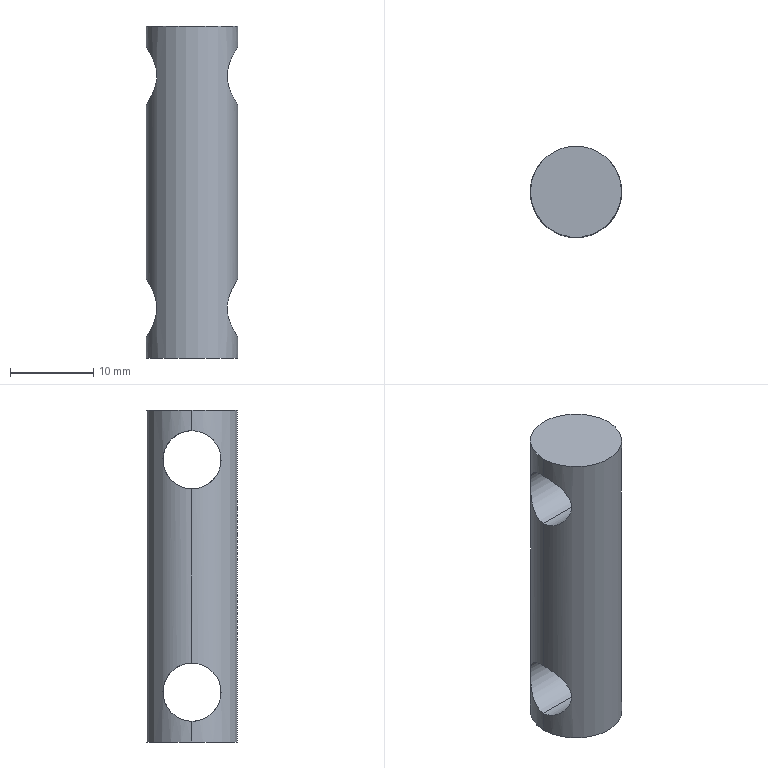Part | SolidWorks | features Extrusion 1, ICE 1 | 1 solid | 8 faces | box 11 x 11 x 40 mm | volume 3000 mm3 | cylinder 6 | plane 2 | commonest cylinder face diameters 7 x4 11 x2
STEP:
#1=CARTESIAN_POINT('',(-5.5,0.,-10.5));
#2=VERTEX_POINT('',#1);
#3=CARTESIAN_POINT('',(-5.5,0.,-17.5));
#4=VERTEX_POINT('',#3);
#5=CARTESIAN_POINT('',(-5.5,0.,-10.5));
#6=CARTESIAN_POINT('',(-5.5,-0.2386,-10.5));
#7=CARTESIAN_POINT('',(-5.485,-0.472,-10.524));
#8=CARTESIAN_POINT('',(-5.426,-0.9292,-10.618));
#9=CARTESIAN_POINT('',(-5.382,-1.155,-10.688));
#10=CARTESIAN_POINT('',(-5.219,-1.788,-10.957));
#11=CARTESIAN_POINT('',(-5.067,-2.167,-11.216));
#12=CARTESIAN_POINT('',(-4.83,-2.636,-11.687));
#13=CARTESIAN_POINT('',(-4.748,-2.779,-11.861));
#14=CARTESIAN_POINT('',(-4.594,-3.028,-12.231));
#15=CARTESIAN_POINT('',(-4.521,-3.134,-12.426));
#16=CARTESIAN_POINT('',(-4.393,-3.311,-12.843));
#17=CARTESIAN_POINT('',(-4.338,-3.381,-13.067));
#18=CARTESIAN_POINT('',(-4.263,-3.475,-13.523));
#19=CARTESIAN_POINT('',(-4.243,-3.5,-13.76));
#20=CARTESIAN_POINT('',(-4.242,-3.5,-14.234));
#21=CARTESIAN_POINT('',(-4.262,-3.477,-14.467));
#22=CARTESIAN_POINT('',(-4.337,-3.383,-14.926));
#23=CARTESIAN_POINT('',(-4.391,-3.314,-15.148));
#24=CARTESIAN_POINT('',(-4.519,-3.137,-15.568));
#25=CARTESIAN_POINT('',(-4.593,-3.029,-15.768));
#26=CARTESIAN_POINT('',(-4.748,-2.78,-16.138));
#27=CARTESIAN_POINT('',(-4.829,-2.639,-16.31));
#28=CARTESIAN_POINT('',(-5.068,-2.165,-16.786));
#29=CARTESIAN_POINT('',(-5.218,-1.794,-17.041));
#30=CARTESIAN_POINT('',(-5.382,-1.155,-17.312));
#31=CARTESIAN_POINT('',(-5.425,-0.9336,-17.381));
#32=CARTESIAN_POINT('',(-5.484,-0.4746,-17.476));
#33=CARTESIAN_POINT('',(-5.5,-0.2353,-17.5));
#34=CARTESIAN_POINT('',(-5.5,0.,-17.5));
#35=B_SPLINE_CURVE_WITH_KNOTS('',3,(#5,#6,#7,#8,#9,#10,#11,#12,#13,#14,#15,#16,#17,#18,#19,#20,#21,#22,#23,#24,#25,#26,#27,#28,#29,#30,#31,#32,#33,#34),.UNSPECIFIED.,.F.,.F.,(4,2,2,2,2,2,2,2,2,2,2,2,2,2,4),(0.,0.0007043,0.001409,0.002817,0.003522,0.004226,0.00493,0.005635,0.006339,0.007043,0.007748,0.008452,0.009861,0.01057,0.01127),.UNSPECIFIED.);
#36=EDGE_CURVE('',#2,#4,#35,.T.);
#37=ORIENTED_EDGE('',*,*,#36,.F.);
#38=CARTESIAN_POINT('',(5.5,0.,-10.5));
#39=VERTEX_POINT('',#38);
#40=CARTESIAN_POINT('',(-20.,0.,-10.5));
#41=DIRECTION('',(1.,0.,0.));
#42=VECTOR('',#41,1000.);
#43=LINE('',#40,#42);
#44=EDGE_CURVE('',#2,#39,#43,.T.);
#45=ORIENTED_EDGE('',*,*,#44,.T.);
#46=CARTESIAN_POINT('',(5.5,0.,-17.5));
#47=VERTEX_POINT('',#46);
#48=CARTESIAN_POINT('',(5.5,0.,-17.5));
#49=CARTESIAN_POINT('',(5.5,-0.2386,-17.5));
#50=CARTESIAN_POINT('',(5.485,-0.472,-17.476));
#51=CARTESIAN_POINT('',(5.426,-0.9292,-17.382));
#52=CARTESIAN_POINT('',(5.382,-1.155,-17.312));
#53=CARTESIAN_POINT('',(5.219,-1.788,-17.043));
#54=CARTESIAN_POINT('',(5.067,-2.167,-16.784));
#55=CARTESIAN_POINT('',(4.83,-2.636,-16.313));
#56=CARTESIAN_POINT('',(4.748,-2.779,-16.139));
#57=CARTESIAN_POINT('',(4.594,-3.028,-15.769));
#58=CARTESIAN_POINT('',(4.521,-3.134,-15.574));
#59=CARTESIAN_POINT('',(4.393,-3.311,-15.157));
#60=CARTESIAN_POINT('',(4.338,-3.381,-14.933));
#61=CARTESIAN_POINT('',(4.263,-3.475,-14.477));
#62=CARTESIAN_POINT('',(4.243,-3.5,-14.24));
#63=CARTESIAN_POINT('',(4.242,-3.5,-13.766));
#64=CARTESIAN_POINT('',(4.262,-3.477,-13.533));
#65=CARTESIAN_POINT('',(4.337,-3.383,-13.074));
#66=CARTESIAN_POINT('',(4.391,-3.314,-12.852));
#67=CARTESIAN_POINT('',(4.519,-3.137,-12.432));
#68=CARTESIAN_POINT('',(4.593,-3.029,-12.232));
#69=CARTESIAN_POINT('',(4.748,-2.78,-11.862));
#70=CARTESIAN_POINT('',(4.829,-2.639,-11.69));
#71=CARTESIAN_POINT('',(5.068,-2.165,-11.214));
#72=CARTESIAN_POINT('',(5.218,-1.794,-10.959));
#73=CARTESIAN_POINT('',(5.382,-1.155,-10.688));
#74=CARTESIAN_POINT('',(5.425,-0.9336,-10.619));
#75=CARTESIAN_POINT('',(5.484,-0.4746,-10.524));
#76=CARTESIAN_POINT('',(5.5,-0.2353,-10.5));
#77=CARTESIAN_POINT('',(5.5,0.,-10.5));
#78=B_SPLINE_CURVE_WITH_KNOTS('',3,(#48,#49,#50,#51,#52,#53,#54,#55,#56,#57,#58,#59,#60,#61,#62,#63,#64,#65,#66,#67,#68,#69,#70,#71,#72,#73,#74,#75,#76,#77),.UNSPECIFIED.,.F.,.F.,(4,2,2,2,2,2,2,2,2,2,2,2,2,2,4),(0.,0.0007043,0.001409,0.002817,0.003522,0.004226,0.00493,0.005635,0.006339,0.007043,0.007748,0.008452,0.009861,0.01057,0.01127),.UNSPECIFIED.);
#79=EDGE_CURVE('',#47,#39,#78,.T.);
#80=ORIENTED_EDGE('',*,*,#79,.F.);
#81=CARTESIAN_POINT('',(-20.,0.,-17.5));
#82=DIRECTION('',(1.,0.,0.));
#83=VECTOR('',#82,1000.);
#84=LINE('',#81,#83);
#85=EDGE_CURVE('',#4,#47,#84,.T.);
#86=ORIENTED_EDGE('',*,*,#85,.F.);
#87=EDGE_LOOP('',(#37,#45,#80,#86));
#88=FACE_OUTER_BOUND('',#87,.T.);
#89=CARTESIAN_POINT('',(-20.,0.,-14.));
#90=DIRECTION('',(1.,0.,0.));
#91=DIRECTION('',(0.,0.,-1.));
#92=AXIS2_PLACEMENT_3D('',#89,#90,#91);
#93=CYLINDRICAL_SURFACE('',#92,3.5);
#94=ADVANCED_FACE('',(#88),#93,.F.);
#95=CARTESIAN_POINT('',(-5.5,0.,17.5));
#96=VERTEX_POINT('',#95);
#97=CARTESIAN_POINT('',(-5.5,0.,10.5));
#98=VERTEX_POINT('',#97);
#99=CARTESIAN_POINT('',(-5.5,0.,17.5));
#100=CARTESIAN_POINT('',(-5.5,-0.2386,17.5));
#101=CARTESIAN_POINT('',(-5.485,-0.472,17.476));
#102=CARTESIAN_POINT('',(-5.426,-0.9292,17.382));
#103=CARTESIAN_POINT('',(-5.382,-1.155,17.312));
#104=CARTESIAN_POINT('',(-5.219,-1.788,17.043));
#105=CARTESIAN_POINT('',(-5.067,-2.167,16.784));
#106=CARTESIAN_POINT('',(-4.83,-2.636,16.313));
#107=CARTESIAN_POINT('',(-4.748,-2.779,16.139));
#108=CARTESIAN_POINT('',(-4.594,-3.028,15.769));
#109=CARTESIAN_POINT('',(-4.521,-3.134,15.574));
#110=CARTESIAN_POINT('',(-4.393,-3.311,15.157));
#111=CARTESIAN_POINT('',(-4.338,-3.381,14.933));
#112=CARTESIAN_POINT('',(-4.263,-3.475,14.477));
#113=CARTESIAN_POINT('',(-4.243,-3.5,14.24));
#114=CARTESIAN_POINT('',(-4.242,-3.5,13.766));
#115=CARTESIAN_POINT('',(-4.262,-3.477,13.533));
#116=CARTESIAN_POINT('',(-4.337,-3.383,13.074));
#117=CARTESIAN_POINT('',(-4.391,-3.314,12.852));
#118=CARTESIAN_POINT('',(-4.519,-3.137,12.432));
#119=CARTESIAN_POINT('',(-4.593,-3.029,12.232));
#120=CARTESIAN_POINT('',(-4.748,-2.78,11.862));
#121=CARTESIAN_POINT('',(-4.829,-2.639,11.69));
#122=CARTESIAN_POINT('',(-5.068,-2.165,11.214));
#123=CARTESIAN_POINT('',(-5.218,-1.794,10.959));
#124=CARTESIAN_POINT('',(-5.382,-1.155,10.688));
#125=CARTESIAN_POINT('',(-5.425,-0.9336,10.619));
#126=CARTESIAN_POINT('',(-5.484,-0.4746,10.524));
#127=CARTESIAN_POINT('',(-5.5,-0.2353,10.5));
#128=CARTESIAN_POINT('',(-5.5,0.,10.5));
#129=B_SPLINE_CURVE_WITH_KNOTS('',3,(#99,#100,#101,#102,#103,#104,#105,#106,#107,#108,#109,#110,#111,#112,#113,#114,#115,#116,#117,#118,#119,#120,#121,#122,#123,#124,#125,#126,#127,#128),.UNSPECIFIED.,.F.,.F.,(4,2,2,2,2,2,2,2,2,2,2,2,2,2,4),(0.,0.0007043,0.001409,0.002817,0.003522,0.004226,0.00493,0.005635,0.006339,0.007043,0.007748,0.008452,0.009861,0.01057,0.01127),.UNSPECIFIED.);
#130=EDGE_CURVE('',#96,#98,#129,.T.);
#131=ORIENTED_EDGE('',*,*,#130,.F.);
#132=CARTESIAN_POINT('',(5.5,0.,17.5));
#133=VERTEX_POINT('',#132);
#134=CARTESIAN_POINT('',(-20.,0.,17.5));
#135=DIRECTION('',(1.,0.,0.));
#136=VECTOR('',#135,1000.);
#137=LINE('',#134,#136);
#138=EDGE_CURVE('',#96,#133,#137,.T.);
#139=ORIENTED_EDGE('',*,*,#138,.T.);
#140=CARTESIAN_POINT('',(5.5,0.,10.5));
#141=VERTEX_POINT('',#140);
#142=CARTESIAN_POINT('',(5.5,0.,10.5));
#143=CARTESIAN_POINT('',(5.5,-0.2386,10.5));
#144=CARTESIAN_POINT('',(5.485,-0.472,10.524));
#145=CARTESIAN_POINT('',(5.426,-0.9292,10.618));
#146=CARTESIAN_POINT('',(5.382,-1.155,10.688));
#147=CARTESIAN_POINT('',(5.219,-1.788,10.957));
#148=CARTESIAN_POINT('',(5.067,-2.167,11.216));
#149=CARTESIAN_POINT('',(4.83,-2.636,11.687));
#150=CARTESIAN_POINT('',(4.748,-2.779,11.861));
#151=CARTESIAN_POINT('',(4.594,-3.028,12.231));
#152=CARTESIAN_POINT('',(4.521,-3.134,12.426));
#153=CARTESIAN_POINT('',(4.393,-3.311,12.843));
#154=CARTESIAN_POINT('',(4.338,-3.381,13.067));
#155=CARTESIAN_POINT('',(4.263,-3.475,13.523));
#156=CARTESIAN_POINT('',(4.243,-3.5,13.76));
#157=CARTESIAN_POINT('',(4.242,-3.5,14.234));
#158=CARTESIAN_POINT('',(4.262,-3.477,14.467));
#159=CARTESIAN_POINT('',(4.337,-3.383,14.926));
#160=CARTESIAN_POINT('',(4.391,-3.314,15.148));
#161=CARTESIAN_POINT('',(4.519,-3.137,15.568));
#162=CARTESIAN_POINT('',(4.593,-3.029,15.768));
#163=CARTESIAN_POINT('',(4.748,-2.78,16.138));
#164=CARTESIAN_POINT('',(4.829,-2.639,16.31));
#165=CARTESIAN_POINT('',(5.068,-2.165,16.786));
#166=CARTESIAN_POINT('',(5.218,-1.794,17.041));
#167=CARTESIAN_POINT('',(5.382,-1.155,17.312));
#168=CARTESIAN_POINT('',(5.425,-0.9336,17.381));
#169=CARTESIAN_POINT('',(5.484,-0.4746,17.476));
#170=CARTESIAN_POINT('',(5.5,-0.2353,17.5));
#171=CARTESIAN_POINT('',(5.5,0.,17.5));
#172=B_SPLINE_CURVE_WITH_KNOTS('',3,(#142,#143,#144,#145,#146,#147,#148,#149,#150,#151,#152,#153,#154,#155,#156,#157,#158,#159,#160,#161,#162,#163,#164,#165,#166,#167,#168,#169,#170,#171),.UNSPECIFIED.,.F.,.F.,(4,2,2,2,2,2,2,2,2,2,2,2,2,2,4),(0.,0.0007043,0.001409,0.002817,0.003522,0.004226,0.00493,0.005635,0.006339,0.007043,0.007748,0.008452,0.009861,0.01057,0.01127),.UNSPECIFIED.);
#173=EDGE_CURVE('',#141,#133,#172,.T.);
#174=ORIENTED_EDGE('',*,*,#173,.F.);
#175=CARTESIAN_POINT('',(-20.,0.,10.5));
#176=DIRECTION('',(1.,0.,0.));
#177=VECTOR('',#176,1000.);
#178=LINE('',#175,#177);
#179=EDGE_CURVE('',#98,#141,#178,.T.);
#180=ORIENTED_EDGE('',*,*,#179,.F.);
#181=EDGE_LOOP('',(#131,#139,#174,#180));
#182=FACE_OUTER_BOUND('',#181,.T.);
#183=CARTESIAN_POINT('',(-20.,0.,14.));
#184=DIRECTION('',(1.,0.,0.));
#185=DIRECTION('',(0.,0.,-1.));
#186=AXIS2_PLACEMENT_3D('',#183,#184,#185);
#187=CYLINDRICAL_SURFACE('',#186,3.5);
#188=ADVANCED_FACE('',(#182),#187,.F.);
#189=CARTESIAN_POINT('',(5.5,0.,20.));
#190=VERTEX_POINT('',#189);
#191=CARTESIAN_POINT('',(-5.5,0.,20.));
#192=VERTEX_POINT('',#191);
#193=CARTESIAN_POINT('',(0.,0.,20.));
#194=DIRECTION('',(0.,0.,1.));
#195=DIRECTION('',(1.,0.,0.));
#196=AXIS2_PLACEMENT_3D('',#193,#194,#195);
#197=CIRCLE('',#196,5.5);
#198=EDGE_CURVE('',#190,#192,#197,.T.);
#199=ORIENTED_EDGE('',*,*,#198,.F.);
#200=CARTESIAN_POINT('',(5.5,0.,20.));
#201=DIRECTION('',(0.,0.,-1.));
#202=VECTOR('',#201,1000.);
#203=LINE('',#200,#202);
#204=EDGE_CURVE('',#190,#133,#203,.T.);
#205=ORIENTED_EDGE('',*,*,#204,.T.);
#206=CARTESIAN_POINT('',(5.5,0.,17.5));
#207=CARTESIAN_POINT('',(5.5,0.235,17.5));
#208=CARTESIAN_POINT('',(5.485,0.4709,17.476));
#209=CARTESIAN_POINT('',(5.425,0.9329,17.382));
#210=CARTESIAN_POINT('',(5.382,1.154,17.312));
#211=CARTESIAN_POINT('',(5.273,1.578,17.133));
#212=CARTESIAN_POINT('',(5.208,1.78,17.022));
#213=CARTESIAN_POINT('',(5.066,2.152,16.77));
#214=CARTESIAN_POINT('',(4.988,2.325,16.626));
#215=CARTESIAN_POINT('',(4.828,2.64,16.309));
#216=CARTESIAN_POINT('',(4.748,2.78,16.138));
#217=CARTESIAN_POINT('',(4.593,3.028,15.769));
#218=CARTESIAN_POINT('',(4.519,3.137,15.568));
#219=CARTESIAN_POINT('',(4.391,3.314,15.15));
#220=CARTESIAN_POINT('',(4.338,3.382,14.931));
#221=CARTESIAN_POINT('',(4.263,3.476,14.47));
#222=CARTESIAN_POINT('',(4.243,3.5,14.236));
#223=CARTESIAN_POINT('',(4.243,3.5,13.766));
#224=CARTESIAN_POINT('',(4.263,3.476,13.527));
#225=CARTESIAN_POINT('',(4.337,3.382,13.07));
#226=CARTESIAN_POINT('',(4.391,3.313,12.849));
#227=CARTESIAN_POINT('',(4.52,3.135,12.427));
#228=CARTESIAN_POINT('',(4.594,3.028,12.231));
#229=CARTESIAN_POINT('',(4.748,2.78,11.862));
#230=CARTESIAN_POINT('',(4.83,2.637,11.688));
#231=CARTESIAN_POINT('',(4.988,2.323,11.373));
#232=CARTESIAN_POINT('',(5.065,2.152,11.231));
#233=CARTESIAN_POINT('',(5.208,1.78,10.978));
#234=CARTESIAN_POINT('',(5.273,1.577,10.867));
#235=CARTESIAN_POINT('',(5.381,1.157,10.689));
#236=CARTESIAN_POINT('',(5.424,0.9374,10.62));
#237=CARTESIAN_POINT('',(5.484,0.4779,10.525));
#238=CARTESIAN_POINT('',(5.5,0.2383,10.5));
#239=CARTESIAN_POINT('',(5.5,0.,10.5));
#240=B_SPLINE_CURVE_WITH_KNOTS('',3,(#206,#207,#208,#209,#210,#211,#212,#213,#214,#215,#216,#217,#218,#219,#220,#221,#222,#223,#224,#225,#226,#227,#228,#229,#230,#231,#232,#233,#234,#235,#236,#237,#238,#239),.UNSPECIFIED.,.F.,.F.,(4,2,2,2,2,2,2,2,2,2,2,2,2,2,2,2,4),(0.01127,0.01197,0.01268,0.01338,0.01408,0.01479,0.01549,0.01619,0.0169,0.0176,0.01831,0.01901,0.01971,0.02042,0.02112,0.02182,0.02253),.UNSPECIFIED.);
#241=EDGE_CURVE('',#133,#141,#240,.T.);
#242=ORIENTED_EDGE('',*,*,#241,.T.);
#243=CARTESIAN_POINT('',(5.5,0.,20.));
#244=DIRECTION('',(0.,0.,-1.));
#245=VECTOR('',#244,1000.);
#246=LINE('',#243,#245);
#247=EDGE_CURVE('',#141,#39,#246,.T.);
#248=ORIENTED_EDGE('',*,*,#247,.T.);
#249=CARTESIAN_POINT('',(5.5,0.,-10.5));
#250=CARTESIAN_POINT('',(5.5,0.235,-10.5));
#251=CARTESIAN_POINT('',(5.485,0.4709,-10.524));
#252=CARTESIAN_POINT('',(5.425,0.9329,-10.618));
#253=CARTESIAN_POINT('',(5.382,1.154,-10.688));
#254=CARTESIAN_POINT('',(5.273,1.578,-10.867));
#255=CARTESIAN_POINT('',(5.208,1.78,-10.978));
#256=CARTESIAN_POINT('',(5.066,2.152,-11.23));
#257=CARTESIAN_POINT('',(4.988,2.325,-11.374));
#258=CARTESIAN_POINT('',(4.828,2.64,-11.691));
#259=CARTESIAN_POINT('',(4.748,2.78,-11.862));
#260=CARTESIAN_POINT('',(4.593,3.028,-12.231));
#261=CARTESIAN_POINT('',(4.519,3.137,-12.432));
#262=CARTESIAN_POINT('',(4.391,3.314,-12.85));
#263=CARTESIAN_POINT('',(4.338,3.382,-13.069));
#264=CARTESIAN_POINT('',(4.263,3.476,-13.53));
#265=CARTESIAN_POINT('',(4.243,3.5,-13.764));
#266=CARTESIAN_POINT('',(4.243,3.5,-14.234));
#267=CARTESIAN_POINT('',(4.263,3.476,-14.473));
#268=CARTESIAN_POINT('',(4.337,3.382,-14.93));
#269=CARTESIAN_POINT('',(4.391,3.313,-15.151));
#270=CARTESIAN_POINT('',(4.52,3.135,-15.573));
#271=CARTESIAN_POINT('',(4.594,3.028,-15.769));
#272=CARTESIAN_POINT('',(4.748,2.78,-16.138));
#273=CARTESIAN_POINT('',(4.83,2.637,-16.312));
#274=CARTESIAN_POINT('',(4.988,2.323,-16.627));
#275=CARTESIAN_POINT('',(5.065,2.152,-16.769));
#276=CARTESIAN_POINT('',(5.208,1.78,-17.022));
#277=CARTESIAN_POINT('',(5.273,1.577,-17.133));
#278=CARTESIAN_POINT('',(5.381,1.157,-17.311));
#279=CARTESIAN_POINT('',(5.424,0.9374,-17.38));
#280=CARTESIAN_POINT('',(5.484,0.4779,-17.475));
#281=CARTESIAN_POINT('',(5.5,0.2383,-17.5));
#282=CARTESIAN_POINT('',(5.5,0.,-17.5));
#283=B_SPLINE_CURVE_WITH_KNOTS('',3,(#249,#250,#251,#252,#253,#254,#255,#256,#257,#258,#259,#260,#261,#262,#263,#264,#265,#266,#267,#268,#269,#270,#271,#272,#273,#274,#275,#276,#277,#278,#279,#280,#281,#282),.UNSPECIFIED.,.F.,.F.,(4,2,2,2,2,2,2,2,2,2,2,2,2,2,2,2,4),(0.01127,0.01197,0.01268,0.01338,0.01408,0.01479,0.01549,0.01619,0.0169,0.0176,0.01831,0.01901,0.01971,0.02042,0.02112,0.02182,0.02253),.UNSPECIFIED.);
#284=EDGE_CURVE('',#39,#47,#283,.T.);
#285=ORIENTED_EDGE('',*,*,#284,.T.);
#286=CARTESIAN_POINT('',(5.5,0.,-20.));
#287=VERTEX_POINT('',#286);
#288=CARTESIAN_POINT('',(5.5,0.,20.));
#289=DIRECTION('',(0.,0.,-1.));
#290=VECTOR('',#289,1000.);
#291=LINE('',#288,#290);
#292=EDGE_CURVE('',#47,#287,#291,.T.);
#293=ORIENTED_EDGE('',*,*,#292,.T.);
#294=CARTESIAN_POINT('',(-5.5,0.,-20.));
#295=VERTEX_POINT('',#294);
#296=CARTESIAN_POINT('',(0.,0.,-20.));
#297=DIRECTION('',(0.,0.,1.));
#298=DIRECTION('',(1.,0.,0.));
#299=AXIS2_PLACEMENT_3D('',#296,#297,#298);
#300=CIRCLE('',#299,5.5);
#301=EDGE_CURVE('',#287,#295,#300,.T.);
#302=ORIENTED_EDGE('',*,*,#301,.T.);
#303=CARTESIAN_POINT('',(-5.5,0.,20.));
#304=DIRECTION('',(0.,0.,-1.));
#305=VECTOR('',#304,1000.);
#306=LINE('',#303,#305);
#307=EDGE_CURVE('',#4,#295,#306,.T.);
#308=ORIENTED_EDGE('',*,*,#307,.F.);
#309=CARTESIAN_POINT('',(-5.5,0.,-17.5));
#310=CARTESIAN_POINT('',(-5.5,0.235,-17.5));
#311=CARTESIAN_POINT('',(-5.485,0.4709,-17.476));
#312=CARTESIAN_POINT('',(-5.425,0.9329,-17.382));
#313=CARTESIAN_POINT('',(-5.382,1.154,-17.312));
#314=CARTESIAN_POINT('',(-5.273,1.578,-17.133));
#315=CARTESIAN_POINT('',(-5.208,1.78,-17.022));
#316=CARTESIAN_POINT('',(-5.066,2.152,-16.77));
#317=CARTESIAN_POINT('',(-4.988,2.325,-16.626));
#318=CARTESIAN_POINT('',(-4.828,2.64,-16.309));
#319=CARTESIAN_POINT('',(-4.748,2.78,-16.138));
#320=CARTESIAN_POINT('',(-4.593,3.028,-15.769));
#321=CARTESIAN_POINT('',(-4.519,3.137,-15.568));
#322=CARTESIAN_POINT('',(-4.391,3.314,-15.15));
#323=CARTESIAN_POINT('',(-4.338,3.382,-14.931));
#324=CARTESIAN_POINT('',(-4.263,3.476,-14.47));
#325=CARTESIAN_POINT('',(-4.243,3.5,-14.236));
#326=CARTESIAN_POINT('',(-4.243,3.5,-13.766));
#327=CARTESIAN_POINT('',(-4.263,3.476,-13.527));
#328=CARTESIAN_POINT('',(-4.337,3.382,-13.07));
#329=CARTESIAN_POINT('',(-4.391,3.313,-12.849));
#330=CARTESIAN_POINT('',(-4.52,3.135,-12.427));
#331=CARTESIAN_POINT('',(-4.594,3.028,-12.231));
#332=CARTESIAN_POINT('',(-4.748,2.78,-11.862));
#333=CARTESIAN_POINT('',(-4.83,2.637,-11.688));
#334=CARTESIAN_POINT('',(-4.988,2.323,-11.373));
#335=CARTESIAN_POINT('',(-5.065,2.152,-11.231));
#336=CARTESIAN_POINT('',(-5.208,1.78,-10.978));
#337=CARTESIAN_POINT('',(-5.273,1.577,-10.867));
#338=CARTESIAN_POINT('',(-5.381,1.157,-10.689));
#339=CARTESIAN_POINT('',(-5.424,0.9374,-10.62));
#340=CARTESIAN_POINT('',(-5.484,0.4779,-10.525));
#341=CARTESIAN_POINT('',(-5.5,0.2383,-10.5));
#342=CARTESIAN_POINT('',(-5.5,0.,-10.5));
#343=B_SPLINE_CURVE_WITH_KNOTS('',3,(#309,#310,#311,#312,#313,#314,#315,#316,#317,#318,#319,#320,#321,#322,#323,#324,#325,#326,#327,#328,#329,#330,#331,#332,#333,#334,#335,#336,#337,#338,#339,#340,#341,#342),.UNSPECIFIED.,.F.,.F.,(4,2,2,2,2,2,2,2,2,2,2,2,2,2,2,2,4),(0.01127,0.01197,0.01268,0.01338,0.01408,0.01479,0.01549,0.01619,0.0169,0.0176,0.01831,0.01901,0.01971,0.02042,0.02112,0.02182,0.02253),.UNSPECIFIED.);
#344=EDGE_CURVE('',#4,#2,#343,.T.);
#345=ORIENTED_EDGE('',*,*,#344,.T.);
#346=CARTESIAN_POINT('',(-5.5,0.,20.));
#347=DIRECTION('',(0.,0.,-1.));
#348=VECTOR('',#347,1000.);
#349=LINE('',#346,#348);
#350=EDGE_CURVE('',#98,#2,#349,.T.);
#351=ORIENTED_EDGE('',*,*,#350,.F.);
#352=CARTESIAN_POINT('',(-5.5,0.,10.5));
#353=CARTESIAN_POINT('',(-5.5,0.235,10.5));
#354=CARTESIAN_POINT('',(-5.485,0.4709,10.524));
#355=CARTESIAN_POINT('',(-5.425,0.9329,10.618));
#356=CARTESIAN_POINT('',(-5.382,1.154,10.688));
#357=CARTESIAN_POINT('',(-5.273,1.578,10.867));
#358=CARTESIAN_POINT('',(-5.208,1.78,10.978));
#359=CARTESIAN_POINT('',(-5.066,2.152,11.23));
#360=CARTESIAN_POINT('',(-4.988,2.325,11.374));
#361=CARTESIAN_POINT('',(-4.828,2.64,11.691));
#362=CARTESIAN_POINT('',(-4.748,2.78,11.862));
#363=CARTESIAN_POINT('',(-4.593,3.028,12.231));
#364=CARTESIAN_POINT('',(-4.519,3.137,12.432));
#365=CARTESIAN_POINT('',(-4.391,3.314,12.85));
#366=CARTESIAN_POINT('',(-4.338,3.382,13.069));
#367=CARTESIAN_POINT('',(-4.263,3.476,13.53));
#368=CARTESIAN_POINT('',(-4.243,3.5,13.764));
#369=CARTESIAN_POINT('',(-4.243,3.5,14.234));
#370=CARTESIAN_POINT('',(-4.263,3.476,14.473));
#371=CARTESIAN_POINT('',(-4.337,3.382,14.93));
#372=CARTESIAN_POINT('',(-4.391,3.313,15.151));
#373=CARTESIAN_POINT('',(-4.52,3.135,15.573));
#374=CARTESIAN_POINT('',(-4.594,3.028,15.769));
#375=CARTESIAN_POINT('',(-4.748,2.78,16.138));
#376=CARTESIAN_POINT('',(-4.83,2.637,16.312));
#377=CARTESIAN_POINT('',(-4.988,2.323,16.627));
#378=CARTESIAN_POINT('',(-5.065,2.152,16.769));
#379=CARTESIAN_POINT('',(-5.208,1.78,17.022));
#380=CARTESIAN_POINT('',(-5.273,1.577,17.133));
#381=CARTESIAN_POINT('',(-5.381,1.157,17.311));
#382=CARTESIAN_POINT('',(-5.424,0.9374,17.38));
#383=CARTESIAN_POINT('',(-5.484,0.4779,17.475));
#384=CARTESIAN_POINT('',(-5.5,0.2383,17.5));
#385=CARTESIAN_POINT('',(-5.5,0.,17.5));
#386=B_SPLINE_CURVE_WITH_KNOTS('',3,(#352,#353,#354,#355,#356,#357,#358,#359,#360,#361,#362,#363,#364,#365,#366,#367,#368,#369,#370,#371,#372,#373,#374,#375,#376,#377,#378,#379,#380,#381,#382,#383,#384,#385),.UNSPECIFIED.,.F.,.F.,(4,2,2,2,2,2,2,2,2,2,2,2,2,2,2,2,4),(0.01127,0.01197,0.01268,0.01338,0.01408,0.01479,0.01549,0.01619,0.0169,0.0176,0.01831,0.01901,0.01971,0.02042,0.02112,0.02182,0.02253),.UNSPECIFIED.);
#387=EDGE_CURVE('',#98,#96,#386,.T.);
#388=ORIENTED_EDGE('',*,*,#387,.T.);
#389=CARTESIAN_POINT('',(-5.5,0.,20.));
#390=DIRECTION('',(0.,0.,-1.));
#391=VECTOR('',#390,1000.);
#392=LINE('',#389,#391);
#393=EDGE_CURVE('',#192,#96,#392,.T.);
#394=ORIENTED_EDGE('',*,*,#393,.F.);
#395=EDGE_LOOP('',(#199,#205,#242,#248,#285,#293,#302,#308,#345,#351,#388,#394));
#396=FACE_OUTER_BOUND('',#395,.T.);
#397=CARTESIAN_POINT('',(0.,0.,20.));
#398=DIRECTION('',(0.,0.,-1.));
#399=DIRECTION('',(-1.,0.,0.));
#400=AXIS2_PLACEMENT_3D('',#397,#398,#399);
#401=CYLINDRICAL_SURFACE('',#400,5.5);
#402=ADVANCED_FACE('',(#396),#401,.T.);
#403=ORIENTED_EDGE('',*,*,#204,.F.);
#404=CARTESIAN_POINT('',(0.,0.,20.));
#405=DIRECTION('',(0.,0.,1.));
#406=DIRECTION('',(1.,0.,0.));
#407=AXIS2_PLACEMENT_3D('',#404,#405,#406);
#408=CIRCLE('',#407,5.5);
#409=EDGE_CURVE('',#192,#190,#408,.T.);
#410=ORIENTED_EDGE('',*,*,#409,.F.);
#411=ORIENTED_EDGE('',*,*,#393,.T.);
#412=ORIENTED_EDGE('',*,*,#130,.T.);
#413=ORIENTED_EDGE('',*,*,#350,.T.);
#414=ORIENTED_EDGE('',*,*,#36,.T.);
#415=ORIENTED_EDGE('',*,*,#307,.T.);
#416=CARTESIAN_POINT('',(0.,0.,-20.));
#417=DIRECTION('',(0.,0.,1.));
#418=DIRECTION('',(1.,0.,0.));
#419=AXIS2_PLACEMENT_3D('',#416,#417,#418);
#420=CIRCLE('',#419,5.5);
#421=EDGE_CURVE('',#295,#287,#420,.T.);
#422=ORIENTED_EDGE('',*,*,#421,.T.);
#423=ORIENTED_EDGE('',*,*,#292,.F.);
#424=ORIENTED_EDGE('',*,*,#79,.T.);
#425=ORIENTED_EDGE('',*,*,#247,.F.);
#426=ORIENTED_EDGE('',*,*,#173,.T.);
#427=EDGE_LOOP('',(#403,#410,#411,#412,#413,#414,#415,#422,#423,#424,#425,#426));
#428=FACE_OUTER_BOUND('',#427,.T.);
#429=CARTESIAN_POINT('',(0.,0.,20.));
#430=DIRECTION('',(0.,0.,-1.));
#431=DIRECTION('',(-1.,0.,0.));
#432=AXIS2_PLACEMENT_3D('',#429,#430,#431);
#433=CYLINDRICAL_SURFACE('',#432,5.5);
#434=ADVANCED_FACE('',(#428),#433,.T.);
#435=ORIENTED_EDGE('',*,*,#409,.T.);
#436=ORIENTED_EDGE('',*,*,#198,.T.);
#437=EDGE_LOOP('',(#435,#436));
#438=FACE_OUTER_BOUND('',#437,.T.);
#439=CARTESIAN_POINT('',(0.,0.,20.));
#440=DIRECTION('',(0.,0.,1.));
#441=DIRECTION('',(1.,0.,0.));
#442=AXIS2_PLACEMENT_3D('',#439,#440,#441);
#443=PLANE('',#442);
#444=ADVANCED_FACE('',(#438),#443,.T.);
#445=ORIENTED_EDGE('',*,*,#421,.F.);
#446=ORIENTED_EDGE('',*,*,#301,.F.);
#447=EDGE_LOOP('',(#445,#446));
#448=FACE_OUTER_BOUND('',#447,.T.);
#449=CARTESIAN_POINT('',(0.,0.,-20.));
#450=DIRECTION('',(0.,0.,1.));
#451=DIRECTION('',(1.,0.,0.));
#452=AXIS2_PLACEMENT_3D('',#449,#450,#451);
#453=PLANE('',#452);
#454=ADVANCED_FACE('',(#448),#453,.F.);
#455=ORIENTED_EDGE('',*,*,#138,.F.);
#456=ORIENTED_EDGE('',*,*,#387,.F.);
#457=ORIENTED_EDGE('',*,*,#179,.T.);
#458=ORIENTED_EDGE('',*,*,#241,.F.);
#459=EDGE_LOOP('',(#455,#456,#457,#458));
#460=FACE_OUTER_BOUND('',#459,.T.);
#461=CARTESIAN_POINT('',(-20.,0.,14.));
#462=DIRECTION('',(1.,0.,0.));
#463=DIRECTION('',(0.,0.,-1.));
#464=AXIS2_PLACEMENT_3D('',#461,#462,#463);
#465=CYLINDRICAL_SURFACE('',#464,3.5);
#466=ADVANCED_FACE('',(#460),#465,.F.);
#467=ORIENTED_EDGE('',*,*,#44,.F.);
#468=ORIENTED_EDGE('',*,*,#344,.F.);
#469=ORIENTED_EDGE('',*,*,#85,.T.);
#470=ORIENTED_EDGE('',*,*,#284,.F.);
#471=EDGE_LOOP('',(#467,#468,#469,#470));
#472=FACE_OUTER_BOUND('',#471,.T.);
#473=CARTESIAN_POINT('',(-20.,0.,-14.));
#474=DIRECTION('',(1.,0.,0.));
#475=DIRECTION('',(0.,0.,-1.));
#476=AXIS2_PLACEMENT_3D('',#473,#474,#475);
#477=CYLINDRICAL_SURFACE('',#476,3.5);
#478=ADVANCED_FACE('',(#472),#477,.F.);
#479=CLOSED_SHELL('',(#94,#188,#402,#434,#444,#454,#466,#478));
#480=MANIFOLD_SOLID_BREP('',#479);
#481=CARTESIAN_POINT('',(0.,0.,0.));
#482=DIRECTION('',(0.,0.,1.));
#483=DIRECTION('',(1.,0.,0.));
#484=AXIS2_PLACEMENT_3D('',#481,#482,#483);
#485=(LENGTH_UNIT()NAMED_UNIT(*)SI_UNIT(.MILLI.,.METRE.));
#486=UNCERTAINTY_MEASURE_WITH_UNIT(LENGTH_MEASURE(0.00001),#485,'','');
#487=(NAMED_UNIT(*)PLANE_ANGLE_UNIT()SI_UNIT($,.RADIAN.));
#488=(NAMED_UNIT(*)SI_UNIT($,.STERADIAN.)SOLID_ANGLE_UNIT());
#489=(GEOMETRIC_REPRESENTATION_CONTEXT(3)GLOBAL_UNCERTAINTY_ASSIGNED_CONTEXT((#486))GLOBAL_UNIT_ASSIGNED_CONTEXT((#485,#487,#488))REPRESENTATION_CONTEXT('',''));
#490=ADVANCED_BREP_SHAPE_REPRESENTATION('',(#480,#484),#489);